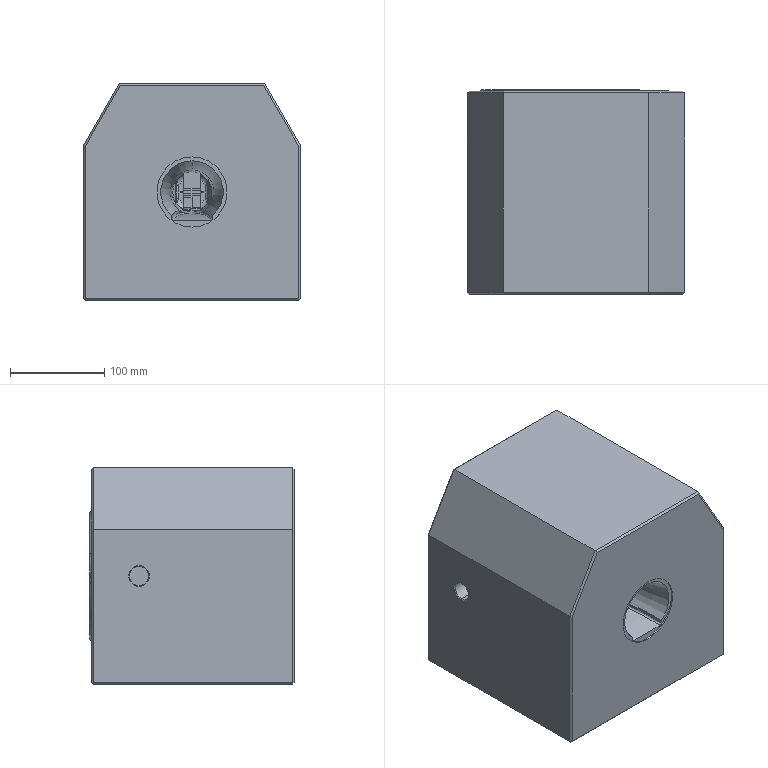Part | STEP file | Cavidade - Torre - 1 cav | 3 solids | 276 faces | box 230 x 216.5 x 230 mm | volume 10150423 mm3 | cylinder 91 | plane 81 | cone 52 | torus 32 | spline 20 | commonest cylinder face diameters 12 x30 10.5 x12 2 x4 3 x4 8 x4 10 x4